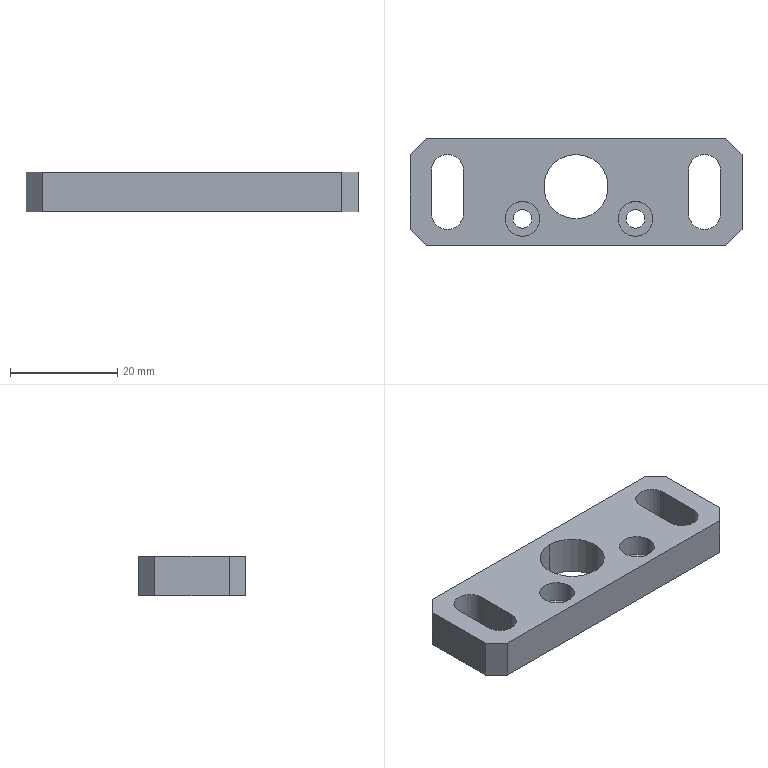Part | STEP file | J454-EBZ05-18-00-Part-1-4 | 1 solid | 30 faces | box 62 x 20 x 7.3 mm | volume 6652 mm3 | plane 16 | cylinder 14 | commonest cylinder face diameters 3.5 x4 6 x4 6.5 x4 12 x2
STEP:
#1=CARTESIAN_POINT('',(-15.,-13.,7.3));
#2=VERTEX_POINT('',#1);
#3=CARTESIAN_POINT('',(-15.,-25.,7.3));
#4=VERTEX_POINT('',#3);
#5=CARTESIAN_POINT('',(-15.,-19.,7.3));
#6=DIRECTION('',(0.,0.,-1.));
#7=DIRECTION('',(0.,-1.,0.));
#8=AXIS2_PLACEMENT_3D('',#5,#6,#7);
#9=CIRCLE('',#8,6.);
#10=EDGE_CURVE('',#2,#4,#9,.T.);
#11=ORIENTED_EDGE('',*,*,#10,.F.);
#12=CARTESIAN_POINT('',(-15.,-13.,0.));
#13=VERTEX_POINT('',#12);
#14=CARTESIAN_POINT('',(-15.,-13.,7.3));
#15=DIRECTION('',(0.,0.,-1.));
#16=VECTOR('',#15,1000.);
#17=LINE('',#14,#16);
#18=EDGE_CURVE('',#2,#13,#17,.T.);
#19=ORIENTED_EDGE('',*,*,#18,.T.);
#20=CARTESIAN_POINT('',(-15.,-25.,0.));
#21=VERTEX_POINT('',#20);
#22=CARTESIAN_POINT('',(-15.,-19.,0.));
#23=DIRECTION('',(0.,0.,1.));
#24=DIRECTION('',(0.,1.,0.));
#25=AXIS2_PLACEMENT_3D('',#22,#23,#24);
#26=CIRCLE('',#25,6.);
#27=EDGE_CURVE('',#21,#13,#26,.T.);
#28=ORIENTED_EDGE('',*,*,#27,.F.);
#29=CARTESIAN_POINT('',(-15.,-25.,7.3));
#30=DIRECTION('',(0.,0.,-1.));
#31=VECTOR('',#30,1000.);
#32=LINE('',#29,#31);
#33=EDGE_CURVE('',#4,#21,#32,.T.);
#34=ORIENTED_EDGE('',*,*,#33,.F.);
#35=EDGE_LOOP('',(#11,#19,#28,#34));
#36=FACE_OUTER_BOUND('',#35,.T.);
#37=CARTESIAN_POINT('',(-15.,-19.,7.3));
#38=DIRECTION('',(0.,0.,-1.));
#39=DIRECTION('',(0.,-1.,0.));
#40=AXIS2_PLACEMENT_3D('',#37,#38,#39);
#41=CYLINDRICAL_SURFACE('',#40,6.);
#42=ADVANCED_FACE('',(#36),#41,.F.);
#43=CARTESIAN_POINT('',(-2.15,-25.,0.));
#44=VERTEX_POINT('',#43);
#45=CARTESIAN_POINT('',(-5.65,-25.,0.));
#46=VERTEX_POINT('',#45);
#47=CARTESIAN_POINT('',(-3.9,-25.,0.));
#48=DIRECTION('',(0.,0.,1.));
#49=DIRECTION('',(-1.,0.,0.));
#50=AXIS2_PLACEMENT_3D('',#47,#48,#49);
#51=CIRCLE('',#50,1.75);
#52=EDGE_CURVE('',#44,#46,#51,.T.);
#53=ORIENTED_EDGE('',*,*,#52,.F.);
#54=CARTESIAN_POINT('',(-2.15,-25.,3.3));
#55=VERTEX_POINT('',#54);
#56=CARTESIAN_POINT('',(-2.15,-25.,7.3));
#57=DIRECTION('',(0.,0.,1.));
#58=VECTOR('',#57,1000.);
#59=LINE('',#56,#58);
#60=EDGE_CURVE('',#44,#55,#59,.T.);
#61=ORIENTED_EDGE('',*,*,#60,.T.);
#62=CARTESIAN_POINT('',(-5.65,-25.,3.3));
#63=VERTEX_POINT('',#62);
#64=CARTESIAN_POINT('',(-3.9,-25.,3.3));
#65=DIRECTION('',(0.,0.,1.));
#66=DIRECTION('',(-1.,0.,0.));
#67=AXIS2_PLACEMENT_3D('',#64,#65,#66);
#68=CIRCLE('',#67,1.75);
#69=EDGE_CURVE('',#55,#63,#68,.T.);
#70=ORIENTED_EDGE('',*,*,#69,.T.);
#71=CARTESIAN_POINT('',(-5.65,-25.,7.3));
#72=DIRECTION('',(0.,0.,1.));
#73=VECTOR('',#72,1000.);
#74=LINE('',#71,#73);
#75=EDGE_CURVE('',#46,#63,#74,.T.);
#76=ORIENTED_EDGE('',*,*,#75,.F.);
#77=EDGE_LOOP('',(#53,#61,#70,#76));
#78=FACE_OUTER_BOUND('',#77,.T.);
#79=CARTESIAN_POINT('',(-3.9,-25.,7.3));
#80=DIRECTION('',(0.,0.,1.));
#81=DIRECTION('',(-1.,0.,0.));
#82=AXIS2_PLACEMENT_3D('',#79,#80,#81);
#83=CYLINDRICAL_SURFACE('',#82,1.75);
#84=ADVANCED_FACE('',(#78),#83,.F.);
#85=CARTESIAN_POINT('',(-0.65,-25.,3.3));
#86=VERTEX_POINT('',#85);
#87=CARTESIAN_POINT('',(-7.15,-25.,3.3));
#88=VERTEX_POINT('',#87);
#89=CARTESIAN_POINT('',(-3.9,-25.,3.3));
#90=DIRECTION('',(0.,0.,1.));
#91=DIRECTION('',(-1.,0.,0.));
#92=AXIS2_PLACEMENT_3D('',#89,#90,#91);
#93=CIRCLE('',#92,3.25);
#94=EDGE_CURVE('',#86,#88,#93,.T.);
#95=ORIENTED_EDGE('',*,*,#94,.F.);
#96=CARTESIAN_POINT('',(-0.65,-25.,7.3));
#97=VERTEX_POINT('',#96);
#98=CARTESIAN_POINT('',(-0.65,-25.,7.3));
#99=DIRECTION('',(0.,0.,1.));
#100=VECTOR('',#99,1000.);
#101=LINE('',#98,#100);
#102=EDGE_CURVE('',#86,#97,#101,.T.);
#103=ORIENTED_EDGE('',*,*,#102,.T.);
#104=CARTESIAN_POINT('',(-7.15,-25.,7.3));
#105=VERTEX_POINT('',#104);
#106=CARTESIAN_POINT('',(-3.9,-25.,7.3));
#107=DIRECTION('',(0.,0.,1.));
#108=DIRECTION('',(-1.,0.,0.));
#109=AXIS2_PLACEMENT_3D('',#106,#107,#108);
#110=CIRCLE('',#109,3.25);
#111=EDGE_CURVE('',#97,#105,#110,.T.);
#112=ORIENTED_EDGE('',*,*,#111,.T.);
#113=CARTESIAN_POINT('',(-7.15,-25.,7.3));
#114=DIRECTION('',(0.,0.,1.));
#115=VECTOR('',#114,1000.);
#116=LINE('',#113,#115);
#117=EDGE_CURVE('',#88,#105,#116,.T.);
#118=ORIENTED_EDGE('',*,*,#117,.F.);
#119=EDGE_LOOP('',(#95,#103,#112,#118));
#120=FACE_OUTER_BOUND('',#119,.T.);
#121=CARTESIAN_POINT('',(-3.9,-25.,7.3));
#122=DIRECTION('',(0.,0.,1.));
#123=DIRECTION('',(-1.,0.,0.));
#124=AXIS2_PLACEMENT_3D('',#121,#122,#123);
#125=CYLINDRICAL_SURFACE('',#124,3.25);
#126=ADVANCED_FACE('',(#120),#125,.F.);
#127=CARTESIAN_POINT('',(-23.25,-25.,0.));
#128=VERTEX_POINT('',#127);
#129=CARTESIAN_POINT('',(-26.75,-25.,0.));
#130=VERTEX_POINT('',#129);
#131=CARTESIAN_POINT('',(-25.,-25.,0.));
#132=DIRECTION('',(0.,0.,1.));
#133=DIRECTION('',(-1.,0.,0.));
#134=AXIS2_PLACEMENT_3D('',#131,#132,#133);
#135=CIRCLE('',#134,1.75);
#136=EDGE_CURVE('',#128,#130,#135,.T.);
#137=ORIENTED_EDGE('',*,*,#136,.F.);
#138=CARTESIAN_POINT('',(-23.25,-25.,3.3));
#139=VERTEX_POINT('',#138);
#140=CARTESIAN_POINT('',(-23.25,-25.,7.3));
#141=DIRECTION('',(0.,0.,1.));
#142=VECTOR('',#141,1000.);
#143=LINE('',#140,#142);
#144=EDGE_CURVE('',#128,#139,#143,.T.);
#145=ORIENTED_EDGE('',*,*,#144,.T.);
#146=CARTESIAN_POINT('',(-26.75,-25.,3.3));
#147=VERTEX_POINT('',#146);
#148=CARTESIAN_POINT('',(-25.,-25.,3.3));
#149=DIRECTION('',(0.,0.,1.));
#150=DIRECTION('',(-1.,0.,0.));
#151=AXIS2_PLACEMENT_3D('',#148,#149,#150);
#152=CIRCLE('',#151,1.75);
#153=EDGE_CURVE('',#139,#147,#152,.T.);
#154=ORIENTED_EDGE('',*,*,#153,.T.);
#155=CARTESIAN_POINT('',(-26.75,-25.,7.3));
#156=DIRECTION('',(0.,0.,1.));
#157=VECTOR('',#156,1000.);
#158=LINE('',#155,#157);
#159=EDGE_CURVE('',#130,#147,#158,.T.);
#160=ORIENTED_EDGE('',*,*,#159,.F.);
#161=EDGE_LOOP('',(#137,#145,#154,#160));
#162=FACE_OUTER_BOUND('',#161,.T.);
#163=CARTESIAN_POINT('',(-25.,-25.,7.3));
#164=DIRECTION('',(0.,0.,1.));
#165=DIRECTION('',(-1.,0.,0.));
#166=AXIS2_PLACEMENT_3D('',#163,#164,#165);
#167=CYLINDRICAL_SURFACE('',#166,1.75);
#168=ADVANCED_FACE('',(#162),#167,.F.);
#169=CARTESIAN_POINT('',(-21.75,-25.,3.3));
#170=VERTEX_POINT('',#169);
#171=CARTESIAN_POINT('',(-28.25,-25.,3.3));
#172=VERTEX_POINT('',#171);
#173=CARTESIAN_POINT('',(-25.,-25.,3.3));
#174=DIRECTION('',(0.,0.,1.));
#175=DIRECTION('',(-1.,0.,0.));
#176=AXIS2_PLACEMENT_3D('',#173,#174,#175);
#177=CIRCLE('',#176,3.25);
#178=EDGE_CURVE('',#170,#172,#177,.T.);
#179=ORIENTED_EDGE('',*,*,#178,.F.);
#180=CARTESIAN_POINT('',(-21.75,-25.,7.3));
#181=VERTEX_POINT('',#180);
#182=CARTESIAN_POINT('',(-21.75,-25.,7.3));
#183=DIRECTION('',(0.,0.,1.));
#184=VECTOR('',#183,1000.);
#185=LINE('',#182,#184);
#186=EDGE_CURVE('',#170,#181,#185,.T.);
#187=ORIENTED_EDGE('',*,*,#186,.T.);
#188=CARTESIAN_POINT('',(-28.25,-25.,7.3));
#189=VERTEX_POINT('',#188);
#190=CARTESIAN_POINT('',(-25.,-25.,7.3));
#191=DIRECTION('',(0.,0.,1.));
#192=DIRECTION('',(-1.,0.,0.));
#193=AXIS2_PLACEMENT_3D('',#190,#191,#192);
#194=CIRCLE('',#193,3.25);
#195=EDGE_CURVE('',#181,#189,#194,.T.);
#196=ORIENTED_EDGE('',*,*,#195,.T.);
#197=CARTESIAN_POINT('',(-28.25,-25.,7.3));
#198=DIRECTION('',(0.,0.,1.));
#199=VECTOR('',#198,1000.);
#200=LINE('',#197,#199);
#201=EDGE_CURVE('',#172,#189,#200,.T.);
#202=ORIENTED_EDGE('',*,*,#201,.F.);
#203=EDGE_LOOP('',(#179,#187,#196,#202));
#204=FACE_OUTER_BOUND('',#203,.T.);
#205=CARTESIAN_POINT('',(-25.,-25.,7.3));
#206=DIRECTION('',(0.,0.,1.));
#207=DIRECTION('',(-1.,0.,0.));
#208=AXIS2_PLACEMENT_3D('',#205,#206,#207);
#209=CYLINDRICAL_SURFACE('',#208,3.25);
#210=ADVANCED_FACE('',(#204),#209,.F.);
#211=CARTESIAN_POINT('',(-15.,-19.,7.3));
#212=DIRECTION('',(0.,0.,-1.));
#213=DIRECTION('',(0.,-1.,0.));
#214=AXIS2_PLACEMENT_3D('',#211,#212,#213);
#215=CIRCLE('',#214,6.);
#216=EDGE_CURVE('',#4,#2,#215,.T.);
#217=ORIENTED_EDGE('',*,*,#216,.T.);
#218=ORIENTED_EDGE('',*,*,#10,.T.);
#219=EDGE_LOOP('',(#217,#218));
#220=FACE_BOUND('',#219,.T.);
#221=CARTESIAN_POINT('',(-3.9,-25.,7.3));
#222=DIRECTION('',(0.,0.,1.));
#223=DIRECTION('',(-1.,0.,0.));
#224=AXIS2_PLACEMENT_3D('',#221,#222,#223);
#225=CIRCLE('',#224,3.25);
#226=EDGE_CURVE('',#105,#97,#225,.T.);
#227=ORIENTED_EDGE('',*,*,#226,.F.);
#228=ORIENTED_EDGE('',*,*,#111,.F.);
#229=EDGE_LOOP('',(#227,#228));
#230=FACE_BOUND('',#229,.T.);
#231=CARTESIAN_POINT('',(-25.,-25.,7.3));
#232=DIRECTION('',(0.,0.,1.));
#233=DIRECTION('',(-1.,0.,0.));
#234=AXIS2_PLACEMENT_3D('',#231,#232,#233);
#235=CIRCLE('',#234,3.25);
#236=EDGE_CURVE('',#189,#181,#235,.T.);
#237=ORIENTED_EDGE('',*,*,#236,.F.);
#238=ORIENTED_EDGE('',*,*,#195,.F.);
#239=EDGE_LOOP('',(#237,#238));
#240=FACE_BOUND('',#239,.T.);
#241=CARTESIAN_POINT('',(16.,-13.,7.3));
#242=VERTEX_POINT('',#241);
#243=CARTESIAN_POINT('',(16.,-27.,7.3));
#244=VERTEX_POINT('',#243);
#245=CARTESIAN_POINT('',(16.,-20.,7.3));
#246=DIRECTION('',(0.,-1.,0.));
#247=VECTOR('',#246,1000.);
#248=LINE('',#245,#247);
#249=EDGE_CURVE('',#242,#244,#248,.T.);
#250=ORIENTED_EDGE('',*,*,#249,.F.);
#251=CARTESIAN_POINT('',(13.,-10.,7.3));
#252=VERTEX_POINT('',#251);
#253=CARTESIAN_POINT('',(4.,-1.,7.3));
#254=DIRECTION('',(-0.7071,0.7071,0.));
#255=VECTOR('',#254,1000.);
#256=LINE('',#253,#255);
#257=EDGE_CURVE('',#242,#252,#256,.T.);
#258=ORIENTED_EDGE('',*,*,#257,.T.);
#259=CARTESIAN_POINT('',(-43.,-10.,7.3));
#260=VERTEX_POINT('',#259);
#261=CARTESIAN_POINT('',(-15.,-10.,7.3));
#262=DIRECTION('',(1.,0.,0.));
#263=VECTOR('',#262,1000.);
#264=LINE('',#261,#263);
#265=EDGE_CURVE('',#260,#252,#264,.T.);
#266=ORIENTED_EDGE('',*,*,#265,.F.);
#267=CARTESIAN_POINT('',(-46.,-13.,7.3));
#268=VERTEX_POINT('',#267);
#269=CARTESIAN_POINT('',(-34.,-1.,7.3));
#270=DIRECTION('',(-0.7071,-0.7071,0.));
#271=VECTOR('',#270,1000.);
#272=LINE('',#269,#271);
#273=EDGE_CURVE('',#260,#268,#272,.T.);
#274=ORIENTED_EDGE('',*,*,#273,.T.);
#275=CARTESIAN_POINT('',(-46.,-27.,7.3));
#276=VERTEX_POINT('',#275);
#277=CARTESIAN_POINT('',(-46.,-20.,7.3));
#278=DIRECTION('',(0.,1.,0.));
#279=VECTOR('',#278,1000.);
#280=LINE('',#277,#279);
#281=EDGE_CURVE('',#276,#268,#280,.T.);
#282=ORIENTED_EDGE('',*,*,#281,.F.);
#283=CARTESIAN_POINT('',(-43.,-30.,7.3));
#284=VERTEX_POINT('',#283);
#285=CARTESIAN_POINT('',(-34.,-39.,7.3));
#286=DIRECTION('',(0.7071,-0.7071,0.));
#287=VECTOR('',#286,1000.);
#288=LINE('',#285,#287);
#289=EDGE_CURVE('',#276,#284,#288,.T.);
#290=ORIENTED_EDGE('',*,*,#289,.T.);
#291=CARTESIAN_POINT('',(13.,-30.,7.3));
#292=VERTEX_POINT('',#291);
#293=CARTESIAN_POINT('',(-15.,-30.,7.3));
#294=DIRECTION('',(-1.,0.,0.));
#295=VECTOR('',#294,1000.);
#296=LINE('',#293,#295);
#297=EDGE_CURVE('',#292,#284,#296,.T.);
#298=ORIENTED_EDGE('',*,*,#297,.F.);
#299=CARTESIAN_POINT('',(4.,-39.,7.3));
#300=DIRECTION('',(0.7071,0.7071,0.));
#301=VECTOR('',#300,1000.);
#302=LINE('',#299,#301);
#303=EDGE_CURVE('',#292,#244,#302,.T.);
#304=ORIENTED_EDGE('',*,*,#303,.T.);
#305=EDGE_LOOP('',(#250,#258,#266,#274,#282,#290,#298,#304));
#306=FACE_OUTER_BOUND('',#305,.T.);
#307=CARTESIAN_POINT('',(12.,-16.,7.3));
#308=VERTEX_POINT('',#307);
#309=CARTESIAN_POINT('',(12.,-24.,7.3));
#310=VERTEX_POINT('',#309);
#311=CARTESIAN_POINT('',(12.,-20.,7.3));
#312=DIRECTION('',(0.,-1.,0.));
#313=VECTOR('',#312,1000.);
#314=LINE('',#311,#313);
#315=EDGE_CURVE('',#308,#310,#314,.T.);
#316=ORIENTED_EDGE('',*,*,#315,.T.);
#317=CARTESIAN_POINT('',(6.,-24.,7.3));
#318=VERTEX_POINT('',#317);
#319=CARTESIAN_POINT('',(9.,-24.,7.3));
#320=DIRECTION('',(0.,0.,-1.));
#321=DIRECTION('',(-1.,0.,0.));
#322=AXIS2_PLACEMENT_3D('',#319,#320,#321);
#323=CIRCLE('',#322,3.);
#324=EDGE_CURVE('',#310,#318,#323,.T.);
#325=ORIENTED_EDGE('',*,*,#324,.T.);
#326=CARTESIAN_POINT('',(6.,-16.,7.3));
#327=VERTEX_POINT('',#326);
#328=CARTESIAN_POINT('',(6.,-20.,7.3));
#329=DIRECTION('',(0.,1.,0.));
#330=VECTOR('',#329,1000.);
#331=LINE('',#328,#330);
#332=EDGE_CURVE('',#318,#327,#331,.T.);
#333=ORIENTED_EDGE('',*,*,#332,.T.);
#334=CARTESIAN_POINT('',(9.,-16.,7.3));
#335=DIRECTION('',(0.,0.,-1.));
#336=DIRECTION('',(-1.,0.,0.));
#337=AXIS2_PLACEMENT_3D('',#334,#335,#336);
#338=CIRCLE('',#337,3.);
#339=EDGE_CURVE('',#327,#308,#338,.T.);
#340=ORIENTED_EDGE('',*,*,#339,.T.);
#341=EDGE_LOOP('',(#316,#325,#333,#340));
#342=FACE_BOUND('',#341,.T.);
#343=CARTESIAN_POINT('',(-36.,-16.,7.3));
#344=VERTEX_POINT('',#343);
#345=CARTESIAN_POINT('',(-36.,-24.,7.3));
#346=VERTEX_POINT('',#345);
#347=CARTESIAN_POINT('',(-36.,-20.,7.3));
#348=DIRECTION('',(0.,-1.,0.));
#349=VECTOR('',#348,1000.);
#350=LINE('',#347,#349);
#351=EDGE_CURVE('',#344,#346,#350,.T.);
#352=ORIENTED_EDGE('',*,*,#351,.T.);
#353=CARTESIAN_POINT('',(-42.,-24.,7.3));
#354=VERTEX_POINT('',#353);
#355=CARTESIAN_POINT('',(-39.,-24.,7.3));
#356=DIRECTION('',(0.,0.,-1.));
#357=DIRECTION('',(-1.,0.,0.));
#358=AXIS2_PLACEMENT_3D('',#355,#356,#357);
#359=CIRCLE('',#358,3.);
#360=EDGE_CURVE('',#346,#354,#359,.T.);
#361=ORIENTED_EDGE('',*,*,#360,.T.);
#362=CARTESIAN_POINT('',(-42.,-16.,7.3));
#363=VERTEX_POINT('',#362);
#364=CARTESIAN_POINT('',(-42.,-20.,7.3));
#365=DIRECTION('',(0.,1.,0.));
#366=VECTOR('',#365,1000.);
#367=LINE('',#364,#366);
#368=EDGE_CURVE('',#354,#363,#367,.T.);
#369=ORIENTED_EDGE('',*,*,#368,.T.);
#370=CARTESIAN_POINT('',(-39.,-16.,7.3));
#371=DIRECTION('',(0.,0.,-1.));
#372=DIRECTION('',(-1.,0.,0.));
#373=AXIS2_PLACEMENT_3D('',#370,#371,#372);
#374=CIRCLE('',#373,3.);
#375=EDGE_CURVE('',#363,#344,#374,.T.);
#376=ORIENTED_EDGE('',*,*,#375,.T.);
#377=EDGE_LOOP('',(#352,#361,#369,#376));
#378=FACE_BOUND('',#377,.T.);
#379=CARTESIAN_POINT('',(-15.,-20.,7.3));
#380=DIRECTION('',(0.,0.,1.));
#381=DIRECTION('',(1.,0.,0.));
#382=AXIS2_PLACEMENT_3D('',#379,#380,#381);
#383=PLANE('',#382);
#384=ADVANCED_FACE('',(#220,#230,#240,#306,#342,#378),#383,.T.);
#385=ORIENTED_EDGE('',*,*,#27,.T.);
#386=CARTESIAN_POINT('',(-15.,-19.,0.));
#387=DIRECTION('',(0.,0.,1.));
#388=DIRECTION('',(0.,1.,0.));
#389=AXIS2_PLACEMENT_3D('',#386,#387,#388);
#390=CIRCLE('',#389,6.);
#391=EDGE_CURVE('',#13,#21,#390,.T.);
#392=ORIENTED_EDGE('',*,*,#391,.T.);
#393=EDGE_LOOP('',(#385,#392));
#394=FACE_BOUND('',#393,.T.);
#395=CARTESIAN_POINT('',(-3.9,-25.,0.));
#396=DIRECTION('',(0.,0.,1.));
#397=DIRECTION('',(-1.,0.,0.));
#398=AXIS2_PLACEMENT_3D('',#395,#396,#397);
#399=CIRCLE('',#398,1.75);
#400=EDGE_CURVE('',#46,#44,#399,.T.);
#401=ORIENTED_EDGE('',*,*,#400,.T.);
#402=ORIENTED_EDGE('',*,*,#52,.T.);
#403=EDGE_LOOP('',(#401,#402));
#404=FACE_BOUND('',#403,.T.);
#405=CARTESIAN_POINT('',(-25.,-25.,0.));
#406=DIRECTION('',(0.,0.,1.));
#407=DIRECTION('',(-1.,0.,0.));
#408=AXIS2_PLACEMENT_3D('',#405,#406,#407);
#409=CIRCLE('',#408,1.75);
#410=EDGE_CURVE('',#130,#128,#409,.T.);
#411=ORIENTED_EDGE('',*,*,#410,.T.);
#412=ORIENTED_EDGE('',*,*,#136,.T.);
#413=EDGE_LOOP('',(#411,#412));
#414=FACE_BOUND('',#413,.T.);
#415=CARTESIAN_POINT('',(-36.,-24.,0.));
#416=VERTEX_POINT('',#415);
#417=CARTESIAN_POINT('',(-42.,-24.,0.));
#418=VERTEX_POINT('',#417);
#419=CARTESIAN_POINT('',(-39.,-24.,0.));
#420=DIRECTION('',(0.,0.,-1.));
#421=DIRECTION('',(-1.,0.,0.));
#422=AXIS2_PLACEMENT_3D('',#419,#420,#421);
#423=CIRCLE('',#422,3.);
#424=EDGE_CURVE('',#416,#418,#423,.T.);
#425=ORIENTED_EDGE('',*,*,#424,.F.);
#426=CARTESIAN_POINT('',(-36.,-16.,0.));
#427=VERTEX_POINT('',#426);
#428=CARTESIAN_POINT('',(-36.,-20.,0.));
#429=DIRECTION('',(0.,-1.,0.));
#430=VECTOR('',#429,1000.);
#431=LINE('',#428,#430);
#432=EDGE_CURVE('',#427,#416,#431,.T.);
#433=ORIENTED_EDGE('',*,*,#432,.F.);
#434=CARTESIAN_POINT('',(-42.,-16.,0.));
#435=VERTEX_POINT('',#434);
#436=CARTESIAN_POINT('',(-39.,-16.,0.));
#437=DIRECTION('',(0.,0.,-1.));
#438=DIRECTION('',(-1.,0.,0.));
#439=AXIS2_PLACEMENT_3D('',#436,#437,#438);
#440=CIRCLE('',#439,3.);
#441=EDGE_CURVE('',#435,#427,#440,.T.);
#442=ORIENTED_EDGE('',*,*,#441,.F.);
#443=CARTESIAN_POINT('',(-42.,-20.,0.));
#444=DIRECTION('',(0.,1.,0.));
#445=VECTOR('',#444,1000.);
#446=LINE('',#443,#445);
#447=EDGE_CURVE('',#418,#435,#446,.T.);
#448=ORIENTED_EDGE('',*,*,#447,.F.);
#449=EDGE_LOOP('',(#425,#433,#442,#448));
#450=FACE_BOUND('',#449,.T.);
#451=CARTESIAN_POINT('',(12.,-24.,0.));
#452=VERTEX_POINT('',#451);
#453=CARTESIAN_POINT('',(6.,-24.,0.));
#454=VERTEX_POINT('',#453);
#455=CARTESIAN_POINT('',(9.,-24.,0.));
#456=DIRECTION('',(0.,0.,-1.));
#457=DIRECTION('',(-1.,0.,0.));
#458=AXIS2_PLACEMENT_3D('',#455,#456,#457);
#459=CIRCLE('',#458,3.);
#460=EDGE_CURVE('',#452,#454,#459,.T.);
#461=ORIENTED_EDGE('',*,*,#460,.F.);
#462=CARTESIAN_POINT('',(12.,-16.,0.));
#463=VERTEX_POINT('',#462);
#464=CARTESIAN_POINT('',(12.,-20.,0.));
#465=DIRECTION('',(0.,-1.,0.));
#466=VECTOR('',#465,1000.);
#467=LINE('',#464,#466);
#468=EDGE_CURVE('',#463,#452,#467,.T.);
#469=ORIENTED_EDGE('',*,*,#468,.F.);
#470=CARTESIAN_POINT('',(6.,-16.,0.));
#471=VERTEX_POINT('',#470);
#472=CARTESIAN_POINT('',(9.,-16.,0.));
#473=DIRECTION('',(0.,0.,-1.));
#474=DIRECTION('',(-1.,0.,0.));
#475=AXIS2_PLACEMENT_3D('',#472,#473,#474);
#476=CIRCLE('',#475,3.);
#477=EDGE_CURVE('',#471,#463,#476,.T.);
#478=ORIENTED_EDGE('',*,*,#477,.F.);
#479=CARTESIAN_POINT('',(6.,-20.,0.));
#480=DIRECTION('',(0.,1.,0.));
#481=VECTOR('',#480,1000.);
#482=LINE('',#479,#481);
#483=EDGE_CURVE('',#454,#471,#482,.T.);
#484=ORIENTED_EDGE('',*,*,#483,.F.);
#485=EDGE_LOOP('',(#461,#469,#478,#484));
#486=FACE_BOUND('',#485,.T.);
#487=CARTESIAN_POINT('',(13.,-10.,0.));
#488=VERTEX_POINT('',#487);
#489=CARTESIAN_POINT('',(-43.,-10.,0.));
#490=VERTEX_POINT('',#489);
#491=CARTESIAN_POINT('',(-15.,-10.,0.));
#492=DIRECTION('',(-1.,0.,0.));
#493=VECTOR('',#492,1000.);
#494=LINE('',#491,#493);
#495=EDGE_CURVE('',#488,#490,#494,.T.);
#496=ORIENTED_EDGE('',*,*,#495,.F.);
#497=CARTESIAN_POINT('',(16.,-13.,0.));
#498=VERTEX_POINT('',#497);
#499=CARTESIAN_POINT('',(4.,-1.,0.));
#500=DIRECTION('',(0.7071,-0.7071,0.));
#501=VECTOR('',#500,1000.);
#502=LINE('',#499,#501);
#503=EDGE_CURVE('',#488,#498,#502,.T.);
#504=ORIENTED_EDGE('',*,*,#503,.T.);
#505=CARTESIAN_POINT('',(16.,-27.,0.));
#506=VERTEX_POINT('',#505);
#507=CARTESIAN_POINT('',(16.,-20.,0.));
#508=DIRECTION('',(0.,1.,0.));
#509=VECTOR('',#508,1000.);
#510=LINE('',#507,#509);
#511=EDGE_CURVE('',#506,#498,#510,.T.);
#512=ORIENTED_EDGE('',*,*,#511,.F.);
#513=CARTESIAN_POINT('',(13.,-30.,0.));
#514=VERTEX_POINT('',#513);
#515=CARTESIAN_POINT('',(4.,-39.,0.));
#516=DIRECTION('',(-0.7071,-0.7071,0.));
#517=VECTOR('',#516,1000.);
#518=LINE('',#515,#517);
#519=EDGE_CURVE('',#506,#514,#518,.T.);
#520=ORIENTED_EDGE('',*,*,#519,.T.);
#521=CARTESIAN_POINT('',(-43.,-30.,0.));
#522=VERTEX_POINT('',#521);
#523=CARTESIAN_POINT('',(-15.,-30.,0.));
#524=DIRECTION('',(1.,0.,0.));
#525=VECTOR('',#524,1000.);
#526=LINE('',#523,#525);
#527=EDGE_CURVE('',#522,#514,#526,.T.);
#528=ORIENTED_EDGE('',*,*,#527,.F.);
#529=CARTESIAN_POINT('',(-46.,-27.,0.));
#530=VERTEX_POINT('',#529);
#531=CARTESIAN_POINT('',(-34.,-39.,0.));
#532=DIRECTION('',(-0.7071,0.7071,0.));
#533=VECTOR('',#532,1000.);
#534=LINE('',#531,#533);
#535=EDGE_CURVE('',#522,#530,#534,.T.);
#536=ORIENTED_EDGE('',*,*,#535,.T.);
#537=CARTESIAN_POINT('',(-46.,-13.,0.));
#538=VERTEX_POINT('',#537);
#539=CARTESIAN_POINT('',(-46.,-20.,0.));
#540=DIRECTION('',(0.,-1.,0.));
#541=VECTOR('',#540,1000.);
#542=LINE('',#539,#541);
#543=EDGE_CURVE('',#538,#530,#542,.T.);
#544=ORIENTED_EDGE('',*,*,#543,.F.);
#545=CARTESIAN_POINT('',(-34.,-1.,0.));
#546=DIRECTION('',(0.7071,0.7071,0.));
#547=VECTOR('',#546,1000.);
#548=LINE('',#545,#547);
#549=EDGE_CURVE('',#538,#490,#548,.T.);
#550=ORIENTED_EDGE('',*,*,#549,.T.);
#551=EDGE_LOOP('',(#496,#504,#512,#520,#528,#536,#544,#550));
#552=FACE_OUTER_BOUND('',#551,.T.);
#553=CARTESIAN_POINT('',(-15.,-20.,0.));
#554=DIRECTION('',(0.,0.,-1.));
#555=DIRECTION('',(-1.,0.,0.));
#556=AXIS2_PLACEMENT_3D('',#553,#554,#555);
#557=PLANE('',#556);
#558=ADVANCED_FACE('',(#394,#404,#414,#450,#486,#552),#557,.T.);
#559=ORIENTED_EDGE('',*,*,#527,.T.);
#560=CARTESIAN_POINT('',(13.,-30.,7.3));
#561=DIRECTION('',(0.,0.,1.));
#562=VECTOR('',#561,1000.);
#563=LINE('',#560,#562);
#564=EDGE_CURVE('',#514,#292,#563,.T.);
#565=ORIENTED_EDGE('',*,*,#564,.T.);
#566=ORIENTED_EDGE('',*,*,#297,.T.);
#567=CARTESIAN_POINT('',(-43.,-30.,7.3));
#568=DIRECTION('',(0.,0.,-1.));
#569=VECTOR('',#568,1000.);
#570=LINE('',#567,#569);
#571=EDGE_CURVE('',#284,#522,#570,.T.);
#572=ORIENTED_EDGE('',*,*,#571,.T.);
#573=EDGE_LOOP('',(#559,#565,#566,#572));
#574=FACE_OUTER_BOUND('',#573,.T.);
#575=CARTESIAN_POINT('',(-15.,-30.,7.3));
#576=DIRECTION('',(0.,-1.,0.));
#577=DIRECTION('',(0.,0.,1.));
#578=AXIS2_PLACEMENT_3D('',#575,#576,#577);
#579=PLANE('',#578);
#580=ADVANCED_FACE('',(#574),#579,.T.);
#581=ORIENTED_EDGE('',*,*,#511,.T.);
#582=CARTESIAN_POINT('',(16.,-13.,7.3));
#583=DIRECTION('',(0.,0.,1.));
#584=VECTOR('',#583,1000.);
#585=LINE('',#582,#584);
#586=EDGE_CURVE('',#498,#242,#585,.T.);
#587=ORIENTED_EDGE('',*,*,#586,.T.);
#588=ORIENTED_EDGE('',*,*,#249,.T.);
#589=CARTESIAN_POINT('',(16.,-27.,7.3));
#590=DIRECTION('',(0.,0.,-1.));
#591=VECTOR('',#590,1000.);
#592=LINE('',#589,#591);
#593=EDGE_CURVE('',#244,#506,#592,.T.);
#594=ORIENTED_EDGE('',*,*,#593,.T.);
#595=EDGE_LOOP('',(#581,#587,#588,#594));
#596=FACE_OUTER_BOUND('',#595,.T.);
#597=CARTESIAN_POINT('',(16.,-20.,7.3));
#598=DIRECTION('',(1.,0.,0.));
#599=DIRECTION('',(0.,0.,-1.));
#600=AXIS2_PLACEMENT_3D('',#597,#598,#599);
#601=PLANE('',#600);
#602=ADVANCED_FACE('',(#596),#601,.T.);
#603=ORIENTED_EDGE('',*,*,#265,.T.);
#604=CARTESIAN_POINT('',(13.,-10.,7.3));
#605=DIRECTION('',(0.,0.,-1.));
#606=VECTOR('',#605,1000.);
#607=LINE('',#604,#606);
#608=EDGE_CURVE('',#252,#488,#607,.T.);
#609=ORIENTED_EDGE('',*,*,#608,.T.);
#610=ORIENTED_EDGE('',*,*,#495,.T.);
#611=CARTESIAN_POINT('',(-43.,-10.,7.3));
#612=DIRECTION('',(0.,0.,1.));
#613=VECTOR('',#612,1000.);
#614=LINE('',#611,#613);
#615=EDGE_CURVE('',#490,#260,#614,.T.);
#616=ORIENTED_EDGE('',*,*,#615,.T.);
#617=EDGE_LOOP('',(#603,#609,#610,#616));
#618=FACE_OUTER_BOUND('',#617,.T.);
#619=CARTESIAN_POINT('',(-15.,-10.,7.3));
#620=DIRECTION('',(0.,1.,0.));
#621=DIRECTION('',(0.,0.,-1.));
#622=AXIS2_PLACEMENT_3D('',#619,#620,#621);
#623=PLANE('',#622);
#624=ADVANCED_FACE('',(#618),#623,.T.);
#625=ORIENTED_EDGE('',*,*,#281,.T.);
#626=CARTESIAN_POINT('',(-46.,-13.,7.3));
#627=DIRECTION('',(0.,0.,-1.));
#628=VECTOR('',#627,1000.);
#629=LINE('',#626,#628);
#630=EDGE_CURVE('',#268,#538,#629,.T.);
#631=ORIENTED_EDGE('',*,*,#630,.T.);
#632=ORIENTED_EDGE('',*,*,#543,.T.);
#633=CARTESIAN_POINT('',(-46.,-27.,7.3));
#634=DIRECTION('',(0.,0.,1.));
#635=VECTOR('',#634,1000.);
#636=LINE('',#633,#635);
#637=EDGE_CURVE('',#530,#276,#636,.T.);
#638=ORIENTED_EDGE('',*,*,#637,.T.);
#639=EDGE_LOOP('',(#625,#631,#632,#638));
#640=FACE_OUTER_BOUND('',#639,.T.);
#641=CARTESIAN_POINT('',(-46.,-20.,7.3));
#642=DIRECTION('',(-1.,0.,0.));
#643=DIRECTION('',(0.,0.,1.));
#644=AXIS2_PLACEMENT_3D('',#641,#642,#643);
#645=PLANE('',#644);
#646=ADVANCED_FACE('',(#640),#645,.T.);
#647=ORIENTED_EDGE('',*,*,#289,.F.);
#648=ORIENTED_EDGE('',*,*,#637,.F.);
#649=ORIENTED_EDGE('',*,*,#535,.F.);
#650=ORIENTED_EDGE('',*,*,#571,.F.);
#651=EDGE_LOOP('',(#647,#648,#649,#650));
#652=FACE_OUTER_BOUND('',#651,.T.);
#653=CARTESIAN_POINT('',(-43.,-30.,7.3));
#654=DIRECTION('',(0.7071,0.7071,0.));
#655=DIRECTION('',(0.,0.,-1.));
#656=AXIS2_PLACEMENT_3D('',#653,#654,#655);
#657=PLANE('',#656);
#658=ADVANCED_FACE('',(#652),#657,.F.);
#659=ORIENTED_EDGE('',*,*,#303,.F.);
#660=ORIENTED_EDGE('',*,*,#564,.F.);
#661=ORIENTED_EDGE('',*,*,#519,.F.);
#662=ORIENTED_EDGE('',*,*,#593,.F.);
#663=EDGE_LOOP('',(#659,#660,#661,#662));
#664=FACE_OUTER_BOUND('',#663,.T.);
#665=CARTESIAN_POINT('',(16.,-27.,7.3));
#666=DIRECTION('',(-0.7071,0.7071,0.));
#667=DIRECTION('',(0.,0.,-1.));
#668=AXIS2_PLACEMENT_3D('',#665,#666,#667);
#669=PLANE('',#668);
#670=ADVANCED_FACE('',(#664),#669,.F.);
#671=ORIENTED_EDGE('',*,*,#468,.T.);
#672=CARTESIAN_POINT('',(12.,-24.,-4.7));
#673=DIRECTION('',(0.,0.,1.));
#674=VECTOR('',#673,1000.);
#675=LINE('',#672,#674);
#676=EDGE_CURVE('',#452,#310,#675,.T.);
#677=ORIENTED_EDGE('',*,*,#676,.T.);
#678=ORIENTED_EDGE('',*,*,#315,.F.);
#679=CARTESIAN_POINT('',(12.,-16.,-4.7));
#680=DIRECTION('',(0.,0.,1.));
#681=VECTOR('',#680,1000.);
#682=LINE('',#679,#681);
#683=EDGE_CURVE('',#463,#308,#682,.T.);
#684=ORIENTED_EDGE('',*,*,#683,.F.);
#685=EDGE_LOOP('',(#671,#677,#678,#684));
#686=FACE_OUTER_BOUND('',#685,.T.);
#687=CARTESIAN_POINT('',(12.,-20.,-4.7));
#688=DIRECTION('',(1.,0.,0.));
#689=DIRECTION('',(0.,0.,-1.));
#690=AXIS2_PLACEMENT_3D('',#687,#688,#689);
#691=PLANE('',#690);
#692=ADVANCED_FACE('',(#686),#691,.F.);
#693=ORIENTED_EDGE('',*,*,#483,.T.);
#694=CARTESIAN_POINT('',(6.,-16.,-4.7));
#695=DIRECTION('',(0.,0.,1.));
#696=VECTOR('',#695,1000.);
#697=LINE('',#694,#696);
#698=EDGE_CURVE('',#471,#327,#697,.T.);
#699=ORIENTED_EDGE('',*,*,#698,.T.);
#700=ORIENTED_EDGE('',*,*,#332,.F.);
#701=CARTESIAN_POINT('',(6.,-24.,-4.7));
#702=DIRECTION('',(0.,0.,1.));
#703=VECTOR('',#702,1000.);
#704=LINE('',#701,#703);
#705=EDGE_CURVE('',#454,#318,#704,.T.);
#706=ORIENTED_EDGE('',*,*,#705,.F.);
#707=EDGE_LOOP('',(#693,#699,#700,#706));
#708=FACE_OUTER_BOUND('',#707,.T.);
#709=CARTESIAN_POINT('',(6.,-20.,-4.7));
#710=DIRECTION('',(-1.,0.,0.));
#711=DIRECTION('',(0.,0.,1.));
#712=AXIS2_PLACEMENT_3D('',#709,#710,#711);
#713=PLANE('',#712);
#714=ADVANCED_FACE('',(#708),#713,.F.);
#715=ORIENTED_EDGE('',*,*,#460,.T.);
#716=ORIENTED_EDGE('',*,*,#705,.T.);
#717=ORIENTED_EDGE('',*,*,#324,.F.);
#718=ORIENTED_EDGE('',*,*,#676,.F.);
#719=EDGE_LOOP('',(#715,#716,#717,#718));
#720=FACE_OUTER_BOUND('',#719,.T.);
#721=CARTESIAN_POINT('',(9.,-24.,-4.7));
#722=DIRECTION('',(0.,0.,1.));
#723=DIRECTION('',(1.,0.,0.));
#724=AXIS2_PLACEMENT_3D('',#721,#722,#723);
#725=CYLINDRICAL_SURFACE('',#724,3.);
#726=ADVANCED_FACE('',(#720),#725,.F.);
#727=ORIENTED_EDGE('',*,*,#477,.T.);
#728=ORIENTED_EDGE('',*,*,#683,.T.);
#729=ORIENTED_EDGE('',*,*,#339,.F.);
#730=ORIENTED_EDGE('',*,*,#698,.F.);
#731=EDGE_LOOP('',(#727,#728,#729,#730));
#732=FACE_OUTER_BOUND('',#731,.T.);
#733=CARTESIAN_POINT('',(9.,-16.,-4.7));
#734=DIRECTION('',(0.,0.,1.));
#735=DIRECTION('',(1.,0.,0.));
#736=AXIS2_PLACEMENT_3D('',#733,#734,#735);
#737=CYLINDRICAL_SURFACE('',#736,3.);
#738=ADVANCED_FACE('',(#732),#737,.F.);
#739=ORIENTED_EDGE('',*,*,#432,.T.);
#740=CARTESIAN_POINT('',(-36.,-24.,-4.7));
#741=DIRECTION('',(0.,0.,1.));
#742=VECTOR('',#741,1000.);
#743=LINE('',#740,#742);
#744=EDGE_CURVE('',#416,#346,#743,.T.);
#745=ORIENTED_EDGE('',*,*,#744,.T.);
#746=ORIENTED_EDGE('',*,*,#351,.F.);
#747=CARTESIAN_POINT('',(-36.,-16.,-4.7));
#748=DIRECTION('',(0.,0.,1.));
#749=VECTOR('',#748,1000.);
#750=LINE('',#747,#749);
#751=EDGE_CURVE('',#427,#344,#750,.T.);
#752=ORIENTED_EDGE('',*,*,#751,.F.);
#753=EDGE_LOOP('',(#739,#745,#746,#752));
#754=FACE_OUTER_BOUND('',#753,.T.);
#755=CARTESIAN_POINT('',(-36.,-20.,-4.7));
#756=DIRECTION('',(1.,0.,0.));
#757=DIRECTION('',(0.,0.,-1.));
#758=AXIS2_PLACEMENT_3D('',#755,#756,#757);
#759=PLANE('',#758);
#760=ADVANCED_FACE('',(#754),#759,.F.);
#761=ORIENTED_EDGE('',*,*,#447,.T.);
#762=CARTESIAN_POINT('',(-42.,-16.,-4.7));
#763=DIRECTION('',(0.,0.,1.));
#764=VECTOR('',#763,1000.);
#765=LINE('',#762,#764);
#766=EDGE_CURVE('',#435,#363,#765,.T.);
#767=ORIENTED_EDGE('',*,*,#766,.T.);
#768=ORIENTED_EDGE('',*,*,#368,.F.);
#769=CARTESIAN_POINT('',(-42.,-24.,-4.7));
#770=DIRECTION('',(0.,0.,1.));
#771=VECTOR('',#770,1000.);
#772=LINE('',#769,#771);
#773=EDGE_CURVE('',#418,#354,#772,.T.);
#774=ORIENTED_EDGE('',*,*,#773,.F.);
#775=EDGE_LOOP('',(#761,#767,#768,#774));
#776=FACE_OUTER_BOUND('',#775,.T.);
#777=CARTESIAN_POINT('',(-42.,-20.,-4.7));
#778=DIRECTION('',(-1.,0.,0.));
#779=DIRECTION('',(0.,0.,1.));
#780=AXIS2_PLACEMENT_3D('',#777,#778,#779);
#781=PLANE('',#780);
#782=ADVANCED_FACE('',(#776),#781,.F.);
#783=ORIENTED_EDGE('',*,*,#424,.T.);
#784=ORIENTED_EDGE('',*,*,#773,.T.);
#785=ORIENTED_EDGE('',*,*,#360,.F.);
#786=ORIENTED_EDGE('',*,*,#744,.F.);
#787=EDGE_LOOP('',(#783,#784,#785,#786));
#788=FACE_OUTER_BOUND('',#787,.T.);
#789=CARTESIAN_POINT('',(-39.,-24.,-4.7));
#790=DIRECTION('',(0.,0.,1.));
#791=DIRECTION('',(1.,0.,0.));
#792=AXIS2_PLACEMENT_3D('',#789,#790,#791);
#793=CYLINDRICAL_SURFACE('',#792,3.);
#794=ADVANCED_FACE('',(#788),#793,.F.);
#795=ORIENTED_EDGE('',*,*,#441,.T.);
#796=ORIENTED_EDGE('',*,*,#751,.T.);
#797=ORIENTED_EDGE('',*,*,#375,.F.);
#798=ORIENTED_EDGE('',*,*,#766,.F.);
#799=EDGE_LOOP('',(#795,#796,#797,#798));
#800=FACE_OUTER_BOUND('',#799,.T.);
#801=CARTESIAN_POINT('',(-39.,-16.,-4.7));
#802=DIRECTION('',(0.,0.,1.));
#803=DIRECTION('',(1.,0.,0.));
#804=AXIS2_PLACEMENT_3D('',#801,#802,#803);
#805=CYLINDRICAL_SURFACE('',#804,3.);
#806=ADVANCED_FACE('',(#800),#805,.F.);
#807=ORIENTED_EDGE('',*,*,#273,.F.);
#808=ORIENTED_EDGE('',*,*,#615,.F.);
#809=ORIENTED_EDGE('',*,*,#549,.F.);
#810=ORIENTED_EDGE('',*,*,#630,.F.);
#811=EDGE_LOOP('',(#807,#808,#809,#810));
#812=FACE_OUTER_BOUND('',#811,.T.);
#813=CARTESIAN_POINT('',(-46.,-13.,7.3));
#814=DIRECTION('',(0.7071,-0.7071,0.));
#815=DIRECTION('',(0.,0.,-1.));
#816=AXIS2_PLACEMENT_3D('',#813,#814,#815);
#817=PLANE('',#816);
#818=ADVANCED_FACE('',(#812),#817,.F.);
#819=ORIENTED_EDGE('',*,*,#257,.F.);
#820=ORIENTED_EDGE('',*,*,#586,.F.);
#821=ORIENTED_EDGE('',*,*,#503,.F.);
#822=ORIENTED_EDGE('',*,*,#608,.F.);
#823=EDGE_LOOP('',(#819,#820,#821,#822));
#824=FACE_OUTER_BOUND('',#823,.T.);
#825=CARTESIAN_POINT('',(13.,-10.,7.3));
#826=DIRECTION('',(-0.7071,-0.7071,0.));
#827=DIRECTION('',(0.,0.,-1.));
#828=AXIS2_PLACEMENT_3D('',#825,#826,#827);
#829=PLANE('',#828);
#830=ADVANCED_FACE('',(#824),#829,.F.);
#831=ORIENTED_EDGE('',*,*,#186,.F.);
#832=CARTESIAN_POINT('',(-25.,-25.,3.3));
#833=DIRECTION('',(0.,0.,1.));
#834=DIRECTION('',(-1.,0.,0.));
#835=AXIS2_PLACEMENT_3D('',#832,#833,#834);
#836=CIRCLE('',#835,3.25);
#837=EDGE_CURVE('',#172,#170,#836,.T.);
#838=ORIENTED_EDGE('',*,*,#837,.F.);
#839=ORIENTED_EDGE('',*,*,#201,.T.);
#840=ORIENTED_EDGE('',*,*,#236,.T.);
#841=EDGE_LOOP('',(#831,#838,#839,#840));
#842=FACE_OUTER_BOUND('',#841,.T.);
#843=CARTESIAN_POINT('',(-25.,-25.,7.3));
#844=DIRECTION('',(0.,0.,1.));
#845=DIRECTION('',(-1.,0.,0.));
#846=AXIS2_PLACEMENT_3D('',#843,#844,#845);
#847=CYLINDRICAL_SURFACE('',#846,3.25);
#848=ADVANCED_FACE('',(#842),#847,.F.);
#849=CARTESIAN_POINT('',(-25.,-25.,3.3));
#850=DIRECTION('',(0.,0.,1.));
#851=DIRECTION('',(-1.,0.,0.));
#852=AXIS2_PLACEMENT_3D('',#849,#850,#851);
#853=CIRCLE('',#852,1.75);
#854=EDGE_CURVE('',#147,#139,#853,.T.);
#855=ORIENTED_EDGE('',*,*,#854,.F.);
#856=ORIENTED_EDGE('',*,*,#153,.F.);
#857=EDGE_LOOP('',(#855,#856));
#858=FACE_BOUND('',#857,.T.);
#859=ORIENTED_EDGE('',*,*,#837,.T.);
#860=ORIENTED_EDGE('',*,*,#178,.T.);
#861=EDGE_LOOP('',(#859,#860));
#862=FACE_OUTER_BOUND('',#861,.T.);
#863=CARTESIAN_POINT('',(-21.75,-25.,3.3));
#864=DIRECTION('',(0.,0.,-1.));
#865=DIRECTION('',(1.,0.,0.));
#866=AXIS2_PLACEMENT_3D('',#863,#864,#865);
#867=PLANE('',#866);
#868=ADVANCED_FACE('',(#858,#862),#867,.F.);
#869=ORIENTED_EDGE('',*,*,#144,.F.);
#870=ORIENTED_EDGE('',*,*,#410,.F.);
#871=ORIENTED_EDGE('',*,*,#159,.T.);
#872=ORIENTED_EDGE('',*,*,#854,.T.);
#873=EDGE_LOOP('',(#869,#870,#871,#872));
#874=FACE_OUTER_BOUND('',#873,.T.);
#875=CARTESIAN_POINT('',(-25.,-25.,7.3));
#876=DIRECTION('',(0.,0.,1.));
#877=DIRECTION('',(-1.,0.,0.));
#878=AXIS2_PLACEMENT_3D('',#875,#876,#877);
#879=CYLINDRICAL_SURFACE('',#878,1.75);
#880=ADVANCED_FACE('',(#874),#879,.F.);
#881=ORIENTED_EDGE('',*,*,#102,.F.);
#882=CARTESIAN_POINT('',(-3.9,-25.,3.3));
#883=DIRECTION('',(0.,0.,1.));
#884=DIRECTION('',(-1.,0.,0.));
#885=AXIS2_PLACEMENT_3D('',#882,#883,#884);
#886=CIRCLE('',#885,3.25);
#887=EDGE_CURVE('',#88,#86,#886,.T.);
#888=ORIENTED_EDGE('',*,*,#887,.F.);
#889=ORIENTED_EDGE('',*,*,#117,.T.);
#890=ORIENTED_EDGE('',*,*,#226,.T.);
#891=EDGE_LOOP('',(#881,#888,#889,#890));
#892=FACE_OUTER_BOUND('',#891,.T.);
#893=CARTESIAN_POINT('',(-3.9,-25.,7.3));
#894=DIRECTION('',(0.,0.,1.));
#895=DIRECTION('',(-1.,0.,0.));
#896=AXIS2_PLACEMENT_3D('',#893,#894,#895);
#897=CYLINDRICAL_SURFACE('',#896,3.25);
#898=ADVANCED_FACE('',(#892),#897,.F.);
#899=CARTESIAN_POINT('',(-3.9,-25.,3.3));
#900=DIRECTION('',(0.,0.,1.));
#901=DIRECTION('',(-1.,0.,0.));
#902=AXIS2_PLACEMENT_3D('',#899,#900,#901);
#903=CIRCLE('',#902,1.75);
#904=EDGE_CURVE('',#63,#55,#903,.T.);
#905=ORIENTED_EDGE('',*,*,#904,.F.);
#906=ORIENTED_EDGE('',*,*,#69,.F.);
#907=EDGE_LOOP('',(#905,#906));
#908=FACE_BOUND('',#907,.T.);
#909=ORIENTED_EDGE('',*,*,#887,.T.);
#910=ORIENTED_EDGE('',*,*,#94,.T.);
#911=EDGE_LOOP('',(#909,#910));
#912=FACE_OUTER_BOUND('',#911,.T.);
#913=CARTESIAN_POINT('',(-0.65,-25.,3.3));
#914=DIRECTION('',(0.,0.,-1.));
#915=DIRECTION('',(1.,0.,0.));
#916=AXIS2_PLACEMENT_3D('',#913,#914,#915);
#917=PLANE('',#916);
#918=ADVANCED_FACE('',(#908,#912),#917,.F.);
#919=ORIENTED_EDGE('',*,*,#60,.F.);
#920=ORIENTED_EDGE('',*,*,#400,.F.);
#921=ORIENTED_EDGE('',*,*,#75,.T.);
#922=ORIENTED_EDGE('',*,*,#904,.T.);
#923=EDGE_LOOP('',(#919,#920,#921,#922));
#924=FACE_OUTER_BOUND('',#923,.T.);
#925=CARTESIAN_POINT('',(-3.9,-25.,7.3));
#926=DIRECTION('',(0.,0.,1.));
#927=DIRECTION('',(-1.,0.,0.));
#928=AXIS2_PLACEMENT_3D('',#925,#926,#927);
#929=CYLINDRICAL_SURFACE('',#928,1.75);
#930=ADVANCED_FACE('',(#924),#929,.F.);
#931=ORIENTED_EDGE('',*,*,#18,.F.);
#932=ORIENTED_EDGE('',*,*,#216,.F.);
#933=ORIENTED_EDGE('',*,*,#33,.T.);
#934=ORIENTED_EDGE('',*,*,#391,.F.);
#935=EDGE_LOOP('',(#931,#932,#933,#934));
#936=FACE_OUTER_BOUND('',#935,.T.);
#937=CARTESIAN_POINT('',(-15.,-19.,7.3));
#938=DIRECTION('',(0.,0.,-1.));
#939=DIRECTION('',(0.,-1.,0.));
#940=AXIS2_PLACEMENT_3D('',#937,#938,#939);
#941=CYLINDRICAL_SURFACE('',#940,6.);
#942=ADVANCED_FACE('',(#936),#941,.F.);
#943=CLOSED_SHELL('',(#42,#84,#126,#168,#210,#384,#558,#580,#602,#624,#646,#658,#670,#692,#714,#726,#738,#760,#782,#794,#806,#818,#830,#848,#868,#880,#898,#918,#930,#942));
#944=MANIFOLD_SOLID_BREP('',#943);
#945=CARTESIAN_POINT('',(0.,0.,0.));
#946=DIRECTION('',(0.,0.,1.));
#947=DIRECTION('',(1.,0.,0.));
#948=AXIS2_PLACEMENT_3D('',#945,#946,#947);
#949=(LENGTH_UNIT()NAMED_UNIT(*)SI_UNIT(.MILLI.,.METRE.));
#950=UNCERTAINTY_MEASURE_WITH_UNIT(LENGTH_MEASURE(0.00001),#949,'','');
#951=(NAMED_UNIT(*)PLANE_ANGLE_UNIT()SI_UNIT($,.RADIAN.));
#952=(NAMED_UNIT(*)SI_UNIT($,.STERADIAN.)SOLID_ANGLE_UNIT());
#953=(GEOMETRIC_REPRESENTATION_CONTEXT(3)GLOBAL_UNCERTAINTY_ASSIGNED_CONTEXT((#950))GLOBAL_UNIT_ASSIGNED_CONTEXT((#949,#951,#952))REPRESENTATION_CONTEXT('',''));
#954=ADVANCED_BREP_SHAPE_REPRESENTATION('',(#944,#948),#953);